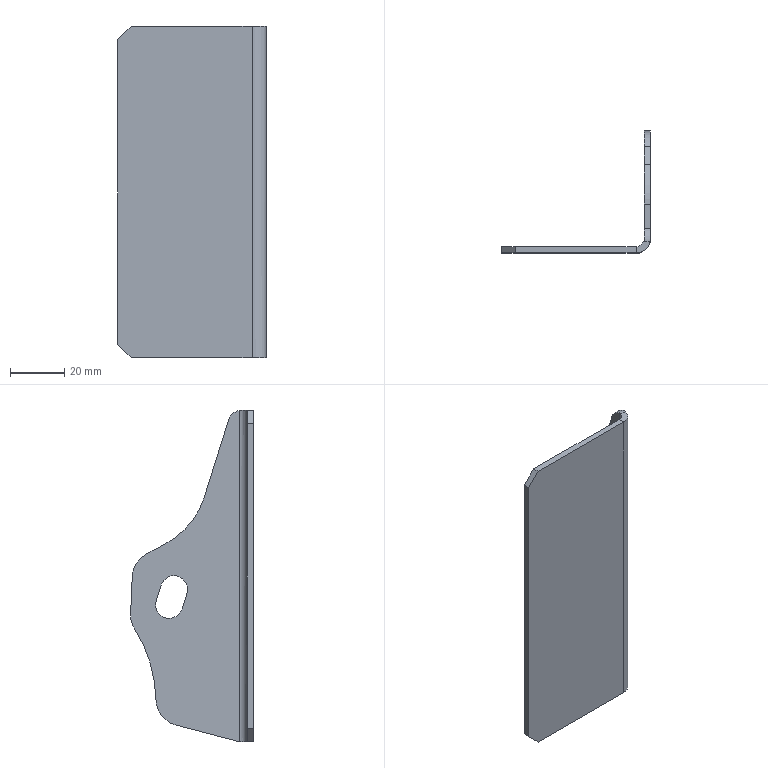Part | SolidWorks | features Chamfer 1, Fillet 1, FlatPattern 1, ICE 1, SMBaseFlange 1, SheetMetal 1 | 1 solid | 29 faces | box 55 x 45.365 x 122.5 mm | volume 22297 mm3 | plane 17 | cylinder 12 | commonest cylinder face diameters 10 x5 20 x3 6 x1 10.6 x1 60 x1 100 x1
STEP:
#1=CARTESIAN_POINT('',(0.,29.298,0.1113));
#2=VERTEX_POINT('',#1);
#3=CARTESIAN_POINT('',(0.,34.067,-3.386));
#4=VERTEX_POINT('',#3);
#5=CARTESIAN_POINT('',(0.,29.298,-4.889));
#6=DIRECTION('',(-1.,0.,0.));
#7=DIRECTION('',(0.,0.,1.));
#8=AXIS2_PLACEMENT_3D('',#5,#6,#7);
#9=CIRCLE('',#8,5.);
#10=EDGE_CURVE('',#2,#4,#9,.T.);
#11=ORIENTED_EDGE('',*,*,#10,.F.);
#12=CARTESIAN_POINT('',(-2.3,29.298,0.1113));
#13=VERTEX_POINT('',#12);
#14=CARTESIAN_POINT('',(-2.3,29.298,0.1113));
#15=DIRECTION('',(-1.,0.,0.));
#16=VECTOR('',#15,1000.);
#17=LINE('',#14,#16);
#18=EDGE_CURVE('',#2,#13,#17,.T.);
#19=ORIENTED_EDGE('',*,*,#18,.T.);
#20=CARTESIAN_POINT('',(-2.3,34.067,-3.386));
#21=VERTEX_POINT('',#20);
#22=CARTESIAN_POINT('',(-2.3,29.298,-4.889));
#23=DIRECTION('',(-1.,0.,0.));
#24=DIRECTION('',(0.,0.,1.));
#25=AXIS2_PLACEMENT_3D('',#22,#23,#24);
#26=CIRCLE('',#25,5.);
#27=EDGE_CURVE('',#13,#21,#26,.T.);
#28=ORIENTED_EDGE('',*,*,#27,.T.);
#29=CARTESIAN_POINT('',(-2.3,34.067,-3.386));
#30=DIRECTION('',(1.,0.,0.));
#31=VECTOR('',#30,1000.);
#32=LINE('',#29,#31);
#33=EDGE_CURVE('',#21,#4,#32,.T.);
#34=ORIENTED_EDGE('',*,*,#33,.T.);
#35=EDGE_LOOP('',(#11,#19,#28,#34));
#36=FACE_OUTER_BOUND('',#35,.T.);
#37=CARTESIAN_POINT('',(-2.3,29.298,-4.889));
#38=DIRECTION('',(-1.,0.,0.));
#39=DIRECTION('',(0.,0.,1.));
#40=AXIS2_PLACEMENT_3D('',#37,#38,#39);
#41=CYLINDRICAL_SURFACE('',#40,5.);
#42=ADVANCED_FACE('',(#36),#41,.F.);
#43=CARTESIAN_POINT('',(-5.3,0.,61.25));
#44=VERTEX_POINT('',#43);
#45=CARTESIAN_POINT('',(-0.08895,4.333,61.25));
#46=VERTEX_POINT('',#45);
#47=CARTESIAN_POINT('',(-5.3,5.3,61.25));
#48=DIRECTION('',(0.,0.,1.));
#49=DIRECTION('',(-1.,0.,0.));
#50=AXIS2_PLACEMENT_3D('',#47,#48,#49);
#51=CIRCLE('',#50,5.3);
#52=EDGE_CURVE('',#44,#46,#51,.T.);
#53=ORIENTED_EDGE('',*,*,#52,.T.);
#54=CARTESIAN_POINT('',(-2.46,4.333,61.25));
#55=VERTEX_POINT('',#54);
#56=CARTESIAN_POINT('',(-5.3,4.333,61.25));
#57=DIRECTION('',(-1.,0.,0.));
#58=VECTOR('',#57,1000.);
#59=LINE('',#56,#58);
#60=EDGE_CURVE('',#46,#55,#59,.T.);
#61=ORIENTED_EDGE('',*,*,#60,.T.);
#62=CARTESIAN_POINT('',(-5.3,2.3,61.25));
#63=VERTEX_POINT('',#62);
#64=CARTESIAN_POINT('',(-5.3,5.3,61.25));
#65=DIRECTION('',(0.,0.,1.));
#66=DIRECTION('',(1.,0.,0.));
#67=AXIS2_PLACEMENT_3D('',#64,#65,#66);
#68=CIRCLE('',#67,3.);
#69=EDGE_CURVE('',#63,#55,#68,.T.);
#70=ORIENTED_EDGE('',*,*,#69,.F.);
#71=CARTESIAN_POINT('',(-5.3,0.,61.25));
#72=DIRECTION('',(0.,1.,0.));
#73=VECTOR('',#72,1000.);
#74=LINE('',#71,#73);
#75=EDGE_CURVE('',#44,#63,#74,.T.);
#76=ORIENTED_EDGE('',*,*,#75,.F.);
#77=EDGE_LOOP('',(#53,#61,#70,#76));
#78=FACE_OUTER_BOUND('',#77,.T.);
#79=CARTESIAN_POINT('',(-5.3,0.,61.25));
#80=DIRECTION('',(0.,0.,1.));
#81=DIRECTION('',(1.,0.,0.));
#82=AXIS2_PLACEMENT_3D('',#79,#80,#81);
#83=PLANE('',#82);
#84=ADVANCED_FACE('',(#78),#83,.T.);
#85=CARTESIAN_POINT('',(-50.,2.3,61.25));
#86=VERTEX_POINT('',#85);
#87=CARTESIAN_POINT('',(0.,2.3,61.25));
#88=DIRECTION('',(1.,0.,0.));
#89=VECTOR('',#88,1000.);
#90=LINE('',#87,#89);
#91=EDGE_CURVE('',#86,#63,#90,.T.);
#92=ORIENTED_EDGE('',*,*,#91,.F.);
#93=CARTESIAN_POINT('',(-50.,0.,61.25));
#94=VERTEX_POINT('',#93);
#95=CARTESIAN_POINT('',(-50.,5.3,61.25));
#96=DIRECTION('',(0.,-1.,0.));
#97=VECTOR('',#96,1000.);
#98=LINE('',#95,#97);
#99=EDGE_CURVE('',#86,#94,#98,.T.);
#100=ORIENTED_EDGE('',*,*,#99,.T.);
#101=CARTESIAN_POINT('',(0.,0.,61.25));
#102=DIRECTION('',(1.,0.,0.));
#103=VECTOR('',#102,1000.);
#104=LINE('',#101,#103);
#105=EDGE_CURVE('',#94,#44,#104,.T.);
#106=ORIENTED_EDGE('',*,*,#105,.T.);
#107=ORIENTED_EDGE('',*,*,#75,.T.);
#108=EDGE_LOOP('',(#92,#100,#106,#107));
#109=FACE_OUTER_BOUND('',#108,.T.);
#110=CARTESIAN_POINT('',(-2.3,5.3,61.25));
#111=DIRECTION('',(0.,0.,1.));
#112=DIRECTION('',(1.,0.,0.));
#113=AXIS2_PLACEMENT_3D('',#110,#111,#112);
#114=PLANE('',#113);
#115=ADVANCED_FACE('',(#109),#114,.T.);
#116=CARTESIAN_POINT('',(-5.3,2.3,-61.25));
#117=VERTEX_POINT('',#116);
#118=CARTESIAN_POINT('',(-2.371,4.652,-61.25));
#119=VERTEX_POINT('',#118);
#120=CARTESIAN_POINT('',(-5.3,5.3,-61.25));
#121=DIRECTION('',(0.,0.,1.));
#122=DIRECTION('',(1.,0.,0.));
#123=AXIS2_PLACEMENT_3D('',#120,#121,#122);
#124=CIRCLE('',#123,3.);
#125=EDGE_CURVE('',#117,#119,#124,.T.);
#126=ORIENTED_EDGE('',*,*,#125,.T.);
#127=CARTESIAN_POINT('',(-0.03977,4.652,-61.25));
#128=VERTEX_POINT('',#127);
#129=CARTESIAN_POINT('',(0.,4.652,-61.25));
#130=DIRECTION('',(1.,0.,0.));
#131=VECTOR('',#130,1000.);
#132=LINE('',#129,#131);
#133=EDGE_CURVE('',#119,#128,#132,.T.);
#134=ORIENTED_EDGE('',*,*,#133,.T.);
#135=CARTESIAN_POINT('',(-5.3,0.,-61.25));
#136=VERTEX_POINT('',#135);
#137=CARTESIAN_POINT('',(-5.3,5.3,-61.25));
#138=DIRECTION('',(0.,0.,1.));
#139=DIRECTION('',(-1.,0.,0.));
#140=AXIS2_PLACEMENT_3D('',#137,#138,#139);
#141=CIRCLE('',#140,5.3);
#142=EDGE_CURVE('',#136,#128,#141,.T.);
#143=ORIENTED_EDGE('',*,*,#142,.F.);
#144=CARTESIAN_POINT('',(-5.3,2.3,-61.25));
#145=DIRECTION('',(0.,-1.,0.));
#146=VECTOR('',#145,1000.);
#147=LINE('',#144,#146);
#148=EDGE_CURVE('',#117,#136,#147,.T.);
#149=ORIENTED_EDGE('',*,*,#148,.F.);
#150=EDGE_LOOP('',(#126,#134,#143,#149));
#151=FACE_OUTER_BOUND('',#150,.T.);
#152=CARTESIAN_POINT('',(0.,5.3,-61.25));
#153=DIRECTION('',(0.,0.,-1.));
#154=DIRECTION('',(-1.,0.,0.));
#155=AXIS2_PLACEMENT_3D('',#152,#153,#154);
#156=PLANE('',#155);
#157=ADVANCED_FACE('',(#151),#156,.T.);
#158=CARTESIAN_POINT('',(0.,5.3,61.156));
#159=VERTEX_POINT('',#158);
#160=CARTESIAN_POINT('',(0.,5.3,-61.208));
#161=VERTEX_POINT('',#160);
#162=CARTESIAN_POINT('',(0.,5.3,61.25));
#163=DIRECTION('',(0.,0.,-1.));
#164=VECTOR('',#163,1000.);
#165=LINE('',#162,#164);
#166=EDGE_CURVE('',#159,#161,#165,.T.);
#167=ORIENTED_EDGE('',*,*,#166,.T.);
#168=CARTESIAN_POINT('',(0.,5.927,-61.085));
#169=VERTEX_POINT('',#168);
#170=CARTESIAN_POINT('',(0.,4.652,-56.25));
#171=DIRECTION('',(1.,0.,0.));
#172=DIRECTION('',(0.,0.,1.));
#173=AXIS2_PLACEMENT_3D('',#170,#171,#172);
#174=CIRCLE('',#173,5.);
#175=EDGE_CURVE('',#161,#169,#174,.T.);
#176=ORIENTED_EDGE('',*,*,#175,.T.);
#177=CARTESIAN_POINT('',(0.,28.542,-55.122));
#178=VERTEX_POINT('',#177);
#179=CARTESIAN_POINT('',(0.,5.3,-61.25));
#180=DIRECTION('',(0.,0.967,0.255));
#181=VECTOR('',#180,1000.);
#182=LINE('',#179,#181);
#183=EDGE_CURVE('',#169,#178,#182,.T.);
#184=ORIENTED_EDGE('',*,*,#183,.T.);
#185=CARTESIAN_POINT('',(0.,35.991,-45.643));
#186=VERTEX_POINT('',#185);
#187=CARTESIAN_POINT('',(0.,25.993,-45.452));
#188=DIRECTION('',(1.,0.,0.));
#189=DIRECTION('',(0.,0.,-1.));
#190=AXIS2_PLACEMENT_3D('',#187,#188,#189);
#191=CIRCLE('',#190,10.);
#192=EDGE_CURVE('',#178,#186,#191,.T.);
#193=ORIENTED_EDGE('',*,*,#192,.T.);
#194=CARTESIAN_POINT('',(0.,43.801,-19.75));
#195=VERTEX_POINT('',#194);
#196=CARTESIAN_POINT('',(0.,85.982,-46.597));
#197=DIRECTION('',(-1.,0.,0.));
#198=DIRECTION('',(0.,0.,1.));
#199=AXIS2_PLACEMENT_3D('',#196,#197,#198);
#200=CIRCLE('',#199,50.);
#201=EDGE_CURVE('',#186,#195,#200,.T.);
#202=ORIENTED_EDGE('',*,*,#201,.T.);
#203=CARTESIAN_POINT('',(0.,45.355,-13.942));
#204=VERTEX_POINT('',#203);
#205=CARTESIAN_POINT('',(0.,35.365,-14.38));
#206=DIRECTION('',(1.,0.,0.));
#207=DIRECTION('',(0.,0.,-1.));
#208=AXIS2_PLACEMENT_3D('',#205,#206,#207);
#209=CIRCLE('',#208,10.);
#210=EDGE_CURVE('',#195,#204,#209,.T.);
#211=ORIENTED_EDGE('',*,*,#210,.T.);
#212=CARTESIAN_POINT('',(0.,44.752,-0.1975));
#213=VERTEX_POINT('',#212);
#214=CARTESIAN_POINT('',(0.,44.752,-0.1975));
#215=DIRECTION('',(0.,-0.04382,0.999));
#216=VECTOR('',#215,1000.);
#217=LINE('',#214,#216);
#218=EDGE_CURVE('',#204,#213,#217,.T.);
#219=ORIENTED_EDGE('',*,*,#218,.T.);
#220=CARTESIAN_POINT('',(0.,39.405,8.221));
#221=VERTEX_POINT('',#220);
#222=CARTESIAN_POINT('',(0.,34.762,-0.6357));
#223=DIRECTION('',(1.,0.,0.));
#224=DIRECTION('',(0.,0.,-1.));
#225=AXIS2_PLACEMENT_3D('',#222,#223,#224);
#226=CIRCLE('',#225,10.);
#227=EDGE_CURVE('',#213,#221,#226,.T.);
#228=ORIENTED_EDGE('',*,*,#227,.T.);
#229=CARTESIAN_POINT('',(0.,32.764,11.702));
#230=VERTEX_POINT('',#229);
#231=CARTESIAN_POINT('',(0.,32.764,11.702));
#232=DIRECTION('',(0.,-0.8857,0.4643));
#233=VECTOR('',#232,1000.);
#234=LINE('',#231,#233);
#235=EDGE_CURVE('',#221,#230,#234,.T.);
#236=ORIENTED_EDGE('',*,*,#235,.T.);
#237=CARTESIAN_POINT('',(0.,18.08,29.257));
#238=VERTEX_POINT('',#237);
#239=CARTESIAN_POINT('',(0.,46.693,38.273));
#240=DIRECTION('',(-1.,0.,0.));
#241=DIRECTION('',(0.,0.,1.));
#242=AXIS2_PLACEMENT_3D('',#239,#240,#241);
#243=CIRCLE('',#242,30.);
#244=EDGE_CURVE('',#230,#238,#243,.T.);
#245=ORIENTED_EDGE('',*,*,#244,.T.);
#246=CARTESIAN_POINT('',(0.,9.102,57.753));
#247=VERTEX_POINT('',#246);
#248=CARTESIAN_POINT('',(0.,18.08,29.257));
#249=DIRECTION('',(0.,-0.3005,0.9538));
#250=VECTOR('',#249,1000.);
#251=LINE('',#248,#250);
#252=EDGE_CURVE('',#238,#247,#251,.T.);
#253=ORIENTED_EDGE('',*,*,#252,.T.);
#254=CARTESIAN_POINT('',(0.,4.333,56.25));
#255=DIRECTION('',(1.,0.,0.));
#256=DIRECTION('',(0.,0.,1.));
#257=AXIS2_PLACEMENT_3D('',#254,#255,#256);
#258=CIRCLE('',#257,5.);
#259=EDGE_CURVE('',#247,#159,#258,.T.);
#260=ORIENTED_EDGE('',*,*,#259,.T.);
#261=EDGE_LOOP('',(#167,#176,#184,#193,#202,#211,#219,#228,#236,#245,#253,#260));
#262=FACE_OUTER_BOUND('',#261,.T.);
#263=CARTESIAN_POINT('',(0.,26.333,-12.114));
#264=VERTEX_POINT('',#263);
#265=CARTESIAN_POINT('',(0.,24.53,-6.391));
#266=VERTEX_POINT('',#265);
#267=CARTESIAN_POINT('',(0.,26.333,-12.114));
#268=DIRECTION('',(0.,-0.3005,0.9538));
#269=VECTOR('',#268,1000.);
#270=LINE('',#267,#269);
#271=EDGE_CURVE('',#264,#266,#270,.T.);
#272=ORIENTED_EDGE('',*,*,#271,.T.);
#273=CARTESIAN_POINT('',(0.,29.298,-4.889));
#274=DIRECTION('',(-1.,0.,0.));
#275=DIRECTION('',(0.,0.,1.));
#276=AXIS2_PLACEMENT_3D('',#273,#274,#275);
#277=CIRCLE('',#276,5.);
#278=EDGE_CURVE('',#266,#2,#277,.T.);
#279=ORIENTED_EDGE('',*,*,#278,.T.);
#280=ORIENTED_EDGE('',*,*,#10,.T.);
#281=CARTESIAN_POINT('',(0.,35.87,-9.109));
#282=VERTEX_POINT('',#281);
#283=CARTESIAN_POINT('',(0.,35.87,-9.109));
#284=DIRECTION('',(0.,0.3005,-0.9538));
#285=VECTOR('',#284,1000.);
#286=LINE('',#283,#285);
#287=EDGE_CURVE('',#4,#282,#286,.T.);
#288=ORIENTED_EDGE('',*,*,#287,.T.);
#289=CARTESIAN_POINT('',(0.,31.102,-10.611));
#290=DIRECTION('',(-1.,0.,0.));
#291=DIRECTION('',(0.,0.,1.));
#292=AXIS2_PLACEMENT_3D('',#289,#290,#291);
#293=CIRCLE('',#292,5.);
#294=EDGE_CURVE('',#282,#264,#293,.T.);
#295=ORIENTED_EDGE('',*,*,#294,.T.);
#296=EDGE_LOOP('',(#272,#279,#280,#288,#295));
#297=FACE_BOUND('',#296,.T.);
#298=CARTESIAN_POINT('',(0.,0.,61.25));
#299=DIRECTION('',(-1.,0.,0.));
#300=DIRECTION('',(0.,0.,1.));
#301=AXIS2_PLACEMENT_3D('',#298,#299,#300);
#302=PLANE('',#301);
#303=ADVANCED_FACE('',(#262,#297),#302,.F.);
#304=CARTESIAN_POINT('',(-2.3,24.53,-6.391));
#305=VERTEX_POINT('',#304);
#306=CARTESIAN_POINT('',(-2.3,29.298,-4.889));
#307=DIRECTION('',(-1.,0.,0.));
#308=DIRECTION('',(0.,0.,1.));
#309=AXIS2_PLACEMENT_3D('',#306,#307,#308);
#310=CIRCLE('',#309,5.);
#311=EDGE_CURVE('',#305,#13,#310,.T.);
#312=ORIENTED_EDGE('',*,*,#311,.F.);
#313=CARTESIAN_POINT('',(-2.3,26.333,-12.114));
#314=VERTEX_POINT('',#313);
#315=CARTESIAN_POINT('',(-2.3,26.333,-12.114));
#316=DIRECTION('',(0.,-0.3005,0.9538));
#317=VECTOR('',#316,1000.);
#318=LINE('',#315,#317);
#319=EDGE_CURVE('',#314,#305,#318,.T.);
#320=ORIENTED_EDGE('',*,*,#319,.F.);
#321=CARTESIAN_POINT('',(-2.3,35.87,-9.109));
#322=VERTEX_POINT('',#321);
#323=CARTESIAN_POINT('',(-2.3,31.102,-10.611));
#324=DIRECTION('',(-1.,0.,0.));
#325=DIRECTION('',(0.,0.,1.));
#326=AXIS2_PLACEMENT_3D('',#323,#324,#325);
#327=CIRCLE('',#326,5.);
#328=EDGE_CURVE('',#322,#314,#327,.T.);
#329=ORIENTED_EDGE('',*,*,#328,.F.);
#330=CARTESIAN_POINT('',(-2.3,35.87,-9.109));
#331=DIRECTION('',(0.,0.3005,-0.9538));
#332=VECTOR('',#331,1000.);
#333=LINE('',#330,#332);
#334=EDGE_CURVE('',#21,#322,#333,.T.);
#335=ORIENTED_EDGE('',*,*,#334,.F.);
#336=ORIENTED_EDGE('',*,*,#27,.F.);
#337=EDGE_LOOP('',(#312,#320,#329,#335,#336));
#338=FACE_BOUND('',#337,.T.);
#339=CARTESIAN_POINT('',(-2.3,5.927,-61.085));
#340=VERTEX_POINT('',#339);
#341=CARTESIAN_POINT('',(-2.3,28.542,-55.122));
#342=VERTEX_POINT('',#341);
#343=CARTESIAN_POINT('',(-2.3,5.3,-61.25));
#344=DIRECTION('',(0.,0.967,0.255));
#345=VECTOR('',#344,1000.);
#346=LINE('',#343,#345);
#347=EDGE_CURVE('',#340,#342,#346,.T.);
#348=ORIENTED_EDGE('',*,*,#347,.F.);
#349=CARTESIAN_POINT('',(-2.3,5.3,-61.208));
#350=VERTEX_POINT('',#349);
#351=CARTESIAN_POINT('',(-2.3,4.652,-56.25));
#352=DIRECTION('',(-1.,0.,0.));
#353=DIRECTION('',(0.,0.,1.));
#354=AXIS2_PLACEMENT_3D('',#351,#352,#353);
#355=CIRCLE('',#354,5.);
#356=EDGE_CURVE('',#340,#350,#355,.T.);
#357=ORIENTED_EDGE('',*,*,#356,.T.);
#358=CARTESIAN_POINT('',(-2.3,5.3,61.156));
#359=VERTEX_POINT('',#358);
#360=CARTESIAN_POINT('',(-2.3,5.3,61.25));
#361=DIRECTION('',(0.,0.,-1.));
#362=VECTOR('',#361,1000.);
#363=LINE('',#360,#362);
#364=EDGE_CURVE('',#359,#350,#363,.T.);
#365=ORIENTED_EDGE('',*,*,#364,.F.);
#366=CARTESIAN_POINT('',(-2.3,9.102,57.753));
#367=VERTEX_POINT('',#366);
#368=CARTESIAN_POINT('',(-2.3,4.333,56.25));
#369=DIRECTION('',(-1.,0.,0.));
#370=DIRECTION('',(0.,0.,1.));
#371=AXIS2_PLACEMENT_3D('',#368,#369,#370);
#372=CIRCLE('',#371,5.);
#373=EDGE_CURVE('',#359,#367,#372,.T.);
#374=ORIENTED_EDGE('',*,*,#373,.T.);
#375=CARTESIAN_POINT('',(-2.3,18.08,29.257));
#376=VERTEX_POINT('',#375);
#377=CARTESIAN_POINT('',(-2.3,18.08,29.257));
#378=DIRECTION('',(0.,-0.3005,0.9538));
#379=VECTOR('',#378,1000.);
#380=LINE('',#377,#379);
#381=EDGE_CURVE('',#376,#367,#380,.T.);
#382=ORIENTED_EDGE('',*,*,#381,.F.);
#383=CARTESIAN_POINT('',(-2.3,32.764,11.702));
#384=VERTEX_POINT('',#383);
#385=CARTESIAN_POINT('',(-2.3,46.693,38.273));
#386=DIRECTION('',(-1.,0.,0.));
#387=DIRECTION('',(0.,0.,1.));
#388=AXIS2_PLACEMENT_3D('',#385,#386,#387);
#389=CIRCLE('',#388,30.);
#390=EDGE_CURVE('',#384,#376,#389,.T.);
#391=ORIENTED_EDGE('',*,*,#390,.F.);
#392=CARTESIAN_POINT('',(-2.3,39.405,8.221));
#393=VERTEX_POINT('',#392);
#394=CARTESIAN_POINT('',(-2.3,32.764,11.702));
#395=DIRECTION('',(0.,-0.8857,0.4643));
#396=VECTOR('',#395,1000.);
#397=LINE('',#394,#396);
#398=EDGE_CURVE('',#393,#384,#397,.T.);
#399=ORIENTED_EDGE('',*,*,#398,.F.);
#400=CARTESIAN_POINT('',(-2.3,44.752,-0.1975));
#401=VERTEX_POINT('',#400);
#402=CARTESIAN_POINT('',(-2.3,34.762,-0.6357));
#403=DIRECTION('',(1.,0.,0.));
#404=DIRECTION('',(0.,0.,-1.));
#405=AXIS2_PLACEMENT_3D('',#402,#403,#404);
#406=CIRCLE('',#405,10.);
#407=EDGE_CURVE('',#401,#393,#406,.T.);
#408=ORIENTED_EDGE('',*,*,#407,.F.);
#409=CARTESIAN_POINT('',(-2.3,45.355,-13.942));
#410=VERTEX_POINT('',#409);
#411=CARTESIAN_POINT('',(-2.3,44.752,-0.1975));
#412=DIRECTION('',(0.,-0.04382,0.999));
#413=VECTOR('',#412,1000.);
#414=LINE('',#411,#413);
#415=EDGE_CURVE('',#410,#401,#414,.T.);
#416=ORIENTED_EDGE('',*,*,#415,.F.);
#417=CARTESIAN_POINT('',(-2.3,43.801,-19.75));
#418=VERTEX_POINT('',#417);
#419=CARTESIAN_POINT('',(-2.3,35.365,-14.38));
#420=DIRECTION('',(1.,0.,0.));
#421=DIRECTION('',(0.,0.,1.));
#422=AXIS2_PLACEMENT_3D('',#419,#420,#421);
#423=CIRCLE('',#422,10.);
#424=EDGE_CURVE('',#418,#410,#423,.T.);
#425=ORIENTED_EDGE('',*,*,#424,.F.);
#426=CARTESIAN_POINT('',(-2.3,35.991,-45.643));
#427=VERTEX_POINT('',#426);
#428=CARTESIAN_POINT('',(-2.3,85.982,-46.597));
#429=DIRECTION('',(-1.,0.,0.));
#430=DIRECTION('',(0.,0.,1.));
#431=AXIS2_PLACEMENT_3D('',#428,#429,#430);
#432=CIRCLE('',#431,50.);
#433=EDGE_CURVE('',#427,#418,#432,.T.);
#434=ORIENTED_EDGE('',*,*,#433,.F.);
#435=CARTESIAN_POINT('',(-2.3,25.993,-45.452));
#436=DIRECTION('',(1.,0.,0.));
#437=DIRECTION('',(0.,0.,-1.));
#438=AXIS2_PLACEMENT_3D('',#435,#436,#437);
#439=CIRCLE('',#438,10.);
#440=EDGE_CURVE('',#342,#427,#439,.T.);
#441=ORIENTED_EDGE('',*,*,#440,.F.);
#442=EDGE_LOOP('',(#348,#357,#365,#374,#382,#391,#399,#408,#416,#425,#434,#441));
#443=FACE_OUTER_BOUND('',#442,.T.);
#444=CARTESIAN_POINT('',(-2.3,0.,61.25));
#445=DIRECTION('',(-1.,0.,0.));
#446=DIRECTION('',(0.,0.,1.));
#447=AXIS2_PLACEMENT_3D('',#444,#445,#446);
#448=PLANE('',#447);
#449=ADVANCED_FACE('',(#338,#443),#448,.T.);
#450=ORIENTED_EDGE('',*,*,#364,.T.);
#451=CARTESIAN_POINT('',(-2.3,5.3,-61.208));
#452=CARTESIAN_POINT('',(-2.3,5.082,-61.236));
#453=CARTESIAN_POINT('',(-2.323,4.866,-61.25));
#454=CARTESIAN_POINT('',(-2.371,4.652,-61.25));
#455=B_SPLINE_CURVE_WITH_KNOTS('',3,(#451,#452,#453,#454),.UNSPECIFIED.,.F.,.F.,(4,4),(0.,0.0006533),.UNSPECIFIED.);
#456=EDGE_CURVE('',#350,#119,#455,.T.);
#457=ORIENTED_EDGE('',*,*,#456,.T.);
#458=ORIENTED_EDGE('',*,*,#125,.F.);
#459=CARTESIAN_POINT('',(-5.3,2.3,61.25));
#460=DIRECTION('',(0.,0.,-1.));
#461=VECTOR('',#460,1000.);
#462=LINE('',#459,#461);
#463=EDGE_CURVE('',#63,#117,#462,.T.);
#464=ORIENTED_EDGE('',*,*,#463,.F.);
#465=ORIENTED_EDGE('',*,*,#69,.T.);
#466=CARTESIAN_POINT('',(-2.46,4.333,61.25));
#467=CARTESIAN_POINT('',(-2.352,4.649,61.25));
#468=CARTESIAN_POINT('',(-2.3,4.972,61.22));
#469=CARTESIAN_POINT('',(-2.3,5.3,61.156));
#470=B_SPLINE_CURVE_WITH_KNOTS('',3,(#466,#467,#468,#469),.UNSPECIFIED.,.F.,.F.,(4,4),(0.,0.0009847),.UNSPECIFIED.);
#471=EDGE_CURVE('',#55,#359,#470,.T.);
#472=ORIENTED_EDGE('',*,*,#471,.T.);
#473=EDGE_LOOP('',(#450,#457,#458,#464,#465,#472));
#474=FACE_OUTER_BOUND('',#473,.T.);
#475=CARTESIAN_POINT('',(-5.3,5.3,61.25));
#476=DIRECTION('',(0.,0.,-1.));
#477=DIRECTION('',(-1.,0.,0.));
#478=AXIS2_PLACEMENT_3D('',#475,#476,#477);
#479=CYLINDRICAL_SURFACE('',#478,3.);
#480=ADVANCED_FACE('',(#474),#479,.F.);
#481=CARTESIAN_POINT('',(-55.,2.3,56.25));
#482=VERTEX_POINT('',#481);
#483=CARTESIAN_POINT('',(-55.,2.3,-56.25));
#484=VERTEX_POINT('',#483);
#485=CARTESIAN_POINT('',(-55.,2.3,61.25));
#486=DIRECTION('',(0.,0.,-1.));
#487=VECTOR('',#486,1000.);
#488=LINE('',#485,#487);
#489=EDGE_CURVE('',#482,#484,#488,.T.);
#490=ORIENTED_EDGE('',*,*,#489,.F.);
#491=CARTESIAN_POINT('',(-25.,2.3,86.25));
#492=DIRECTION('',(0.7071,0.,0.7071));
#493=VECTOR('',#492,1000.);
#494=LINE('',#491,#493);
#495=EDGE_CURVE('',#482,#86,#494,.T.);
#496=ORIENTED_EDGE('',*,*,#495,.T.);
#497=ORIENTED_EDGE('',*,*,#91,.T.);
#498=ORIENTED_EDGE('',*,*,#463,.T.);
#499=CARTESIAN_POINT('',(-50.,2.3,-61.25));
#500=VERTEX_POINT('',#499);
#501=CARTESIAN_POINT('',(0.,2.3,-61.25));
#502=DIRECTION('',(1.,0.,0.));
#503=VECTOR('',#502,1000.);
#504=LINE('',#501,#503);
#505=EDGE_CURVE('',#500,#117,#504,.T.);
#506=ORIENTED_EDGE('',*,*,#505,.F.);
#507=CARTESIAN_POINT('',(-86.25,2.3,-25.));
#508=DIRECTION('',(-0.7071,0.,0.7071));
#509=VECTOR('',#508,1000.);
#510=LINE('',#507,#509);
#511=EDGE_CURVE('',#500,#484,#510,.T.);
#512=ORIENTED_EDGE('',*,*,#511,.T.);
#513=EDGE_LOOP('',(#490,#496,#497,#498,#506,#512));
#514=FACE_OUTER_BOUND('',#513,.T.);
#515=CARTESIAN_POINT('',(0.,2.3,61.25));
#516=DIRECTION('',(0.,1.,0.));
#517=DIRECTION('',(-1.,0.,0.));
#518=AXIS2_PLACEMENT_3D('',#515,#516,#517);
#519=PLANE('',#518);
#520=ADVANCED_FACE('',(#514),#519,.T.);
#521=CARTESIAN_POINT('',(-55.,0.,56.25));
#522=VERTEX_POINT('',#521);
#523=CARTESIAN_POINT('',(-55.,0.,-56.25));
#524=VERTEX_POINT('',#523);
#525=CARTESIAN_POINT('',(-55.,0.,61.25));
#526=DIRECTION('',(0.,0.,-1.));
#527=VECTOR('',#526,1000.);
#528=LINE('',#525,#527);
#529=EDGE_CURVE('',#522,#524,#528,.T.);
#530=ORIENTED_EDGE('',*,*,#529,.F.);
#531=CARTESIAN_POINT('',(-55.,0.,56.25));
#532=DIRECTION('',(0.,1.,0.));
#533=VECTOR('',#532,1000.);
#534=LINE('',#531,#533);
#535=EDGE_CURVE('',#522,#482,#534,.T.);
#536=ORIENTED_EDGE('',*,*,#535,.T.);
#537=ORIENTED_EDGE('',*,*,#489,.T.);
#538=CARTESIAN_POINT('',(-55.,0.,-56.25));
#539=DIRECTION('',(0.,-1.,0.));
#540=VECTOR('',#539,1000.);
#541=LINE('',#538,#540);
#542=EDGE_CURVE('',#484,#524,#541,.T.);
#543=ORIENTED_EDGE('',*,*,#542,.T.);
#544=EDGE_LOOP('',(#530,#536,#537,#543));
#545=FACE_OUTER_BOUND('',#544,.T.);
#546=CARTESIAN_POINT('',(-55.,0.,61.25));
#547=DIRECTION('',(-1.,0.,0.));
#548=DIRECTION('',(0.,0.,1.));
#549=AXIS2_PLACEMENT_3D('',#546,#547,#548);
#550=PLANE('',#549);
#551=ADVANCED_FACE('',(#545),#550,.T.);
#552=ORIENTED_EDGE('',*,*,#105,.F.);
#553=CARTESIAN_POINT('',(-55.,0.,56.25));
#554=DIRECTION('',(-0.7071,0.,-0.7071));
#555=VECTOR('',#554,1000.);
#556=LINE('',#553,#555);
#557=EDGE_CURVE('',#94,#522,#556,.T.);
#558=ORIENTED_EDGE('',*,*,#557,.T.);
#559=ORIENTED_EDGE('',*,*,#529,.T.);
#560=CARTESIAN_POINT('',(-50.,0.,-61.25));
#561=VERTEX_POINT('',#560);
#562=CARTESIAN_POINT('',(-50.,0.,-61.25));
#563=DIRECTION('',(0.7071,0.,-0.7071));
#564=VECTOR('',#563,1000.);
#565=LINE('',#562,#564);
#566=EDGE_CURVE('',#524,#561,#565,.T.);
#567=ORIENTED_EDGE('',*,*,#566,.T.);
#568=CARTESIAN_POINT('',(0.,0.,-61.25));
#569=DIRECTION('',(1.,0.,0.));
#570=VECTOR('',#569,1000.);
#571=LINE('',#568,#570);
#572=EDGE_CURVE('',#561,#136,#571,.T.);
#573=ORIENTED_EDGE('',*,*,#572,.T.);
#574=CARTESIAN_POINT('',(-5.3,0.,61.25));
#575=DIRECTION('',(0.,0.,-1.));
#576=VECTOR('',#575,1000.);
#577=LINE('',#574,#576);
#578=EDGE_CURVE('',#44,#136,#577,.T.);
#579=ORIENTED_EDGE('',*,*,#578,.F.);
#580=EDGE_LOOP('',(#552,#558,#559,#567,#573,#579));
#581=FACE_OUTER_BOUND('',#580,.T.);
#582=CARTESIAN_POINT('',(0.,0.,61.25));
#583=DIRECTION('',(0.,1.,0.));
#584=DIRECTION('',(-1.,0.,0.));
#585=AXIS2_PLACEMENT_3D('',#582,#583,#584);
#586=PLANE('',#585);
#587=ADVANCED_FACE('',(#581),#586,.F.);
#588=ORIENTED_EDGE('',*,*,#142,.T.);
#589=CARTESIAN_POINT('',(-0.03977,4.652,-61.25));
#590=CARTESIAN_POINT('',(-0.01315,4.868,-61.25));
#591=CARTESIAN_POINT('',(0.,5.084,-61.236));
#592=CARTESIAN_POINT('',(0.,5.3,-61.208));
#593=B_SPLINE_CURVE_WITH_KNOTS('',3,(#589,#590,#591,#592),.UNSPECIFIED.,.F.,.F.,(4,4),(0.,0.0006507),.UNSPECIFIED.);
#594=EDGE_CURVE('',#128,#161,#593,.T.);
#595=ORIENTED_EDGE('',*,*,#594,.T.);
#596=ORIENTED_EDGE('',*,*,#166,.F.);
#597=CARTESIAN_POINT('',(0.,5.3,61.156));
#598=CARTESIAN_POINT('',(0.,4.978,61.219));
#599=CARTESIAN_POINT('',(-0.02909,4.656,61.25));
#600=CARTESIAN_POINT('',(-0.08895,4.333,61.25));
#601=B_SPLINE_CURVE_WITH_KNOTS('',3,(#597,#598,#599,#600),.UNSPECIFIED.,.F.,.F.,(4,4),(0.,0.0009756),.UNSPECIFIED.);
#602=EDGE_CURVE('',#159,#46,#601,.T.);
#603=ORIENTED_EDGE('',*,*,#602,.T.);
#604=ORIENTED_EDGE('',*,*,#52,.F.);
#605=ORIENTED_EDGE('',*,*,#578,.T.);
#606=EDGE_LOOP('',(#588,#595,#596,#603,#604,#605));
#607=FACE_OUTER_BOUND('',#606,.T.);
#608=CARTESIAN_POINT('',(-5.3,5.3,61.25));
#609=DIRECTION('',(0.,0.,-1.));
#610=DIRECTION('',(-1.,0.,0.));
#611=AXIS2_PLACEMENT_3D('',#608,#609,#610);
#612=CYLINDRICAL_SURFACE('',#611,5.3);
#613=ADVANCED_FACE('',(#607),#612,.T.);
#614=ORIENTED_EDGE('',*,*,#572,.F.);
#615=CARTESIAN_POINT('',(-50.,2.3,-61.25));
#616=DIRECTION('',(0.,1.,0.));
#617=VECTOR('',#616,1000.);
#618=LINE('',#615,#617);
#619=EDGE_CURVE('',#561,#500,#618,.T.);
#620=ORIENTED_EDGE('',*,*,#619,.T.);
#621=ORIENTED_EDGE('',*,*,#505,.T.);
#622=ORIENTED_EDGE('',*,*,#148,.T.);
#623=EDGE_LOOP('',(#614,#620,#621,#622));
#624=FACE_OUTER_BOUND('',#623,.T.);
#625=CARTESIAN_POINT('',(-5.3,5.3,-61.25));
#626=DIRECTION('',(0.,0.,1.));
#627=DIRECTION('',(1.,0.,0.));
#628=AXIS2_PLACEMENT_3D('',#625,#626,#627);
#629=PLANE('',#628);
#630=ADVANCED_FACE('',(#624),#629,.F.);
#631=ORIENTED_EDGE('',*,*,#183,.F.);
#632=CARTESIAN_POINT('',(-2.3,5.927,-61.085));
#633=DIRECTION('',(-1.,0.,0.));
#634=VECTOR('',#633,1000.);
#635=LINE('',#632,#634);
#636=EDGE_CURVE('',#169,#340,#635,.T.);
#637=ORIENTED_EDGE('',*,*,#636,.T.);
#638=ORIENTED_EDGE('',*,*,#347,.T.);
#639=CARTESIAN_POINT('',(-2.3,28.542,-55.122));
#640=DIRECTION('',(1.,0.,0.));
#641=VECTOR('',#640,1000.);
#642=LINE('',#639,#641);
#643=EDGE_CURVE('',#342,#178,#642,.T.);
#644=ORIENTED_EDGE('',*,*,#643,.T.);
#645=EDGE_LOOP('',(#631,#637,#638,#644));
#646=FACE_OUTER_BOUND('',#645,.T.);
#647=CARTESIAN_POINT('',(-2.3,5.3,-61.25));
#648=DIRECTION('',(0.,-0.255,0.967));
#649=DIRECTION('',(0.,0.967,0.255));
#650=AXIS2_PLACEMENT_3D('',#647,#648,#649);
#651=PLANE('',#650);
#652=ADVANCED_FACE('',(#646),#651,.F.);
#653=ORIENTED_EDGE('',*,*,#643,.F.);
#654=ORIENTED_EDGE('',*,*,#440,.T.);
#655=CARTESIAN_POINT('',(-2.3,35.991,-45.643));
#656=DIRECTION('',(1.,0.,0.));
#657=VECTOR('',#656,1000.);
#658=LINE('',#655,#657);
#659=EDGE_CURVE('',#427,#186,#658,.T.);
#660=ORIENTED_EDGE('',*,*,#659,.T.);
#661=ORIENTED_EDGE('',*,*,#192,.F.);
#662=EDGE_LOOP('',(#653,#654,#660,#661));
#663=FACE_OUTER_BOUND('',#662,.T.);
#664=CARTESIAN_POINT('',(-2.3,25.993,-45.452));
#665=DIRECTION('',(-1.,0.,0.));
#666=DIRECTION('',(0.,0.,1.));
#667=AXIS2_PLACEMENT_3D('',#664,#665,#666);
#668=CYLINDRICAL_SURFACE('',#667,10.);
#669=ADVANCED_FACE('',(#663),#668,.T.);
#670=ORIENTED_EDGE('',*,*,#659,.F.);
#671=ORIENTED_EDGE('',*,*,#433,.T.);
#672=CARTESIAN_POINT('',(-2.3,43.801,-19.75));
#673=DIRECTION('',(1.,0.,0.));
#674=VECTOR('',#673,1000.);
#675=LINE('',#672,#674);
#676=EDGE_CURVE('',#418,#195,#675,.T.);
#677=ORIENTED_EDGE('',*,*,#676,.T.);
#678=ORIENTED_EDGE('',*,*,#201,.F.);
#679=EDGE_LOOP('',(#670,#671,#677,#678));
#680=FACE_OUTER_BOUND('',#679,.T.);
#681=CARTESIAN_POINT('',(-2.3,85.982,-46.597));
#682=DIRECTION('',(-1.,0.,0.));
#683=DIRECTION('',(0.,0.,1.));
#684=AXIS2_PLACEMENT_3D('',#681,#682,#683);
#685=CYLINDRICAL_SURFACE('',#684,50.);
#686=ADVANCED_FACE('',(#680),#685,.F.);
#687=ORIENTED_EDGE('',*,*,#676,.F.);
#688=ORIENTED_EDGE('',*,*,#424,.T.);
#689=CARTESIAN_POINT('',(-2.3,45.355,-13.942));
#690=DIRECTION('',(1.,0.,0.));
#691=VECTOR('',#690,1000.);
#692=LINE('',#689,#691);
#693=EDGE_CURVE('',#410,#204,#692,.T.);
#694=ORIENTED_EDGE('',*,*,#693,.T.);
#695=ORIENTED_EDGE('',*,*,#210,.F.);
#696=EDGE_LOOP('',(#687,#688,#694,#695));
#697=FACE_OUTER_BOUND('',#696,.T.);
#698=CARTESIAN_POINT('',(-2.3,35.365,-14.38));
#699=DIRECTION('',(-1.,0.,0.));
#700=DIRECTION('',(0.,0.,1.));
#701=AXIS2_PLACEMENT_3D('',#698,#699,#700);
#702=CYLINDRICAL_SURFACE('',#701,10.);
#703=ADVANCED_FACE('',(#697),#702,.T.);
#704=ORIENTED_EDGE('',*,*,#693,.F.);
#705=ORIENTED_EDGE('',*,*,#415,.T.);
#706=CARTESIAN_POINT('',(-2.3,44.752,-0.1975));
#707=DIRECTION('',(1.,0.,0.));
#708=VECTOR('',#707,1000.);
#709=LINE('',#706,#708);
#710=EDGE_CURVE('',#401,#213,#709,.T.);
#711=ORIENTED_EDGE('',*,*,#710,.T.);
#712=ORIENTED_EDGE('',*,*,#218,.F.);
#713=EDGE_LOOP('',(#704,#705,#711,#712));
#714=FACE_OUTER_BOUND('',#713,.T.);
#715=CARTESIAN_POINT('',(-2.3,44.752,-0.1975));
#716=DIRECTION('',(0.,-0.999,-0.04382));
#717=DIRECTION('',(0.,-0.04382,0.999));
#718=AXIS2_PLACEMENT_3D('',#715,#716,#717);
#719=PLANE('',#718);
#720=ADVANCED_FACE('',(#714),#719,.F.);
#721=ORIENTED_EDGE('',*,*,#710,.F.);
#722=ORIENTED_EDGE('',*,*,#407,.T.);
#723=CARTESIAN_POINT('',(-2.3,39.405,8.221));
#724=DIRECTION('',(1.,0.,0.));
#725=VECTOR('',#724,1000.);
#726=LINE('',#723,#725);
#727=EDGE_CURVE('',#393,#221,#726,.T.);
#728=ORIENTED_EDGE('',*,*,#727,.T.);
#729=ORIENTED_EDGE('',*,*,#227,.F.);
#730=EDGE_LOOP('',(#721,#722,#728,#729));
#731=FACE_OUTER_BOUND('',#730,.T.);
#732=CARTESIAN_POINT('',(-2.3,34.762,-0.6357));
#733=DIRECTION('',(-1.,0.,0.));
#734=DIRECTION('',(0.,0.,1.));
#735=AXIS2_PLACEMENT_3D('',#732,#733,#734);
#736=CYLINDRICAL_SURFACE('',#735,10.);
#737=ADVANCED_FACE('',(#731),#736,.T.);
#738=ORIENTED_EDGE('',*,*,#727,.F.);
#739=ORIENTED_EDGE('',*,*,#398,.T.);
#740=CARTESIAN_POINT('',(-2.3,32.764,11.702));
#741=DIRECTION('',(1.,0.,0.));
#742=VECTOR('',#741,1000.);
#743=LINE('',#740,#742);
#744=EDGE_CURVE('',#384,#230,#743,.T.);
#745=ORIENTED_EDGE('',*,*,#744,.T.);
#746=ORIENTED_EDGE('',*,*,#235,.F.);
#747=EDGE_LOOP('',(#738,#739,#745,#746));
#748=FACE_OUTER_BOUND('',#747,.T.);
#749=CARTESIAN_POINT('',(-2.3,32.764,11.702));
#750=DIRECTION('',(0.,-0.4643,-0.8857));
#751=DIRECTION('',(0.,-0.8857,0.4643));
#752=AXIS2_PLACEMENT_3D('',#749,#750,#751);
#753=PLANE('',#752);
#754=ADVANCED_FACE('',(#748),#753,.F.);
#755=ORIENTED_EDGE('',*,*,#744,.F.);
#756=ORIENTED_EDGE('',*,*,#390,.T.);
#757=CARTESIAN_POINT('',(-2.3,18.08,29.257));
#758=DIRECTION('',(1.,0.,0.));
#759=VECTOR('',#758,1000.);
#760=LINE('',#757,#759);
#761=EDGE_CURVE('',#376,#238,#760,.T.);
#762=ORIENTED_EDGE('',*,*,#761,.T.);
#763=ORIENTED_EDGE('',*,*,#244,.F.);
#764=EDGE_LOOP('',(#755,#756,#762,#763));
#765=FACE_OUTER_BOUND('',#764,.T.);
#766=CARTESIAN_POINT('',(-2.3,46.693,38.273));
#767=DIRECTION('',(-1.,0.,0.));
#768=DIRECTION('',(0.,0.,1.));
#769=AXIS2_PLACEMENT_3D('',#766,#767,#768);
#770=CYLINDRICAL_SURFACE('',#769,30.);
#771=ADVANCED_FACE('',(#765),#770,.F.);
#772=ORIENTED_EDGE('',*,*,#381,.T.);
#773=CARTESIAN_POINT('',(-2.3,9.102,57.753));
#774=DIRECTION('',(1.,0.,0.));
#775=VECTOR('',#774,1000.);
#776=LINE('',#773,#775);
#777=EDGE_CURVE('',#367,#247,#776,.T.);
#778=ORIENTED_EDGE('',*,*,#777,.T.);
#779=ORIENTED_EDGE('',*,*,#252,.F.);
#780=ORIENTED_EDGE('',*,*,#761,.F.);
#781=EDGE_LOOP('',(#772,#778,#779,#780));
#782=FACE_OUTER_BOUND('',#781,.T.);
#783=CARTESIAN_POINT('',(-2.3,18.08,29.257));
#784=DIRECTION('',(0.,-0.9538,-0.3005));
#785=DIRECTION('',(0.,-0.3005,0.9538));
#786=AXIS2_PLACEMENT_3D('',#783,#784,#785);
#787=PLANE('',#786);
#788=ADVANCED_FACE('',(#782),#787,.F.);
#789=CARTESIAN_POINT('',(-2.3,26.333,-12.114));
#790=DIRECTION('',(1.,0.,0.));
#791=VECTOR('',#790,1000.);
#792=LINE('',#789,#791);
#793=EDGE_CURVE('',#314,#264,#792,.T.);
#794=ORIENTED_EDGE('',*,*,#793,.F.);
#795=ORIENTED_EDGE('',*,*,#319,.T.);
#796=CARTESIAN_POINT('',(-2.3,24.53,-6.391));
#797=DIRECTION('',(1.,0.,0.));
#798=VECTOR('',#797,1000.);
#799=LINE('',#796,#798);
#800=EDGE_CURVE('',#305,#266,#799,.T.);
#801=ORIENTED_EDGE('',*,*,#800,.T.);
#802=ORIENTED_EDGE('',*,*,#271,.F.);
#803=EDGE_LOOP('',(#794,#795,#801,#802));
#804=FACE_OUTER_BOUND('',#803,.T.);
#805=CARTESIAN_POINT('',(-2.3,26.333,-12.114));
#806=DIRECTION('',(0.,-0.9538,-0.3005));
#807=DIRECTION('',(0.,-0.3005,0.9538));
#808=AXIS2_PLACEMENT_3D('',#805,#806,#807);
#809=PLANE('',#808);
#810=ADVANCED_FACE('',(#804),#809,.F.);
#811=ORIENTED_EDGE('',*,*,#18,.F.);
#812=ORIENTED_EDGE('',*,*,#278,.F.);
#813=ORIENTED_EDGE('',*,*,#800,.F.);
#814=ORIENTED_EDGE('',*,*,#311,.T.);
#815=EDGE_LOOP('',(#811,#812,#813,#814));
#816=FACE_OUTER_BOUND('',#815,.T.);
#817=CARTESIAN_POINT('',(-2.3,29.298,-4.889));
#818=DIRECTION('',(-1.,0.,0.));
#819=DIRECTION('',(0.,0.,1.));
#820=AXIS2_PLACEMENT_3D('',#817,#818,#819);
#821=CYLINDRICAL_SURFACE('',#820,5.);
#822=ADVANCED_FACE('',(#816),#821,.F.);
#823=ORIENTED_EDGE('',*,*,#33,.F.);
#824=ORIENTED_EDGE('',*,*,#334,.T.);
#825=CARTESIAN_POINT('',(-2.3,35.87,-9.109));
#826=DIRECTION('',(1.,0.,0.));
#827=VECTOR('',#826,1000.);
#828=LINE('',#825,#827);
#829=EDGE_CURVE('',#322,#282,#828,.T.);
#830=ORIENTED_EDGE('',*,*,#829,.T.);
#831=ORIENTED_EDGE('',*,*,#287,.F.);
#832=EDGE_LOOP('',(#823,#824,#830,#831));
#833=FACE_OUTER_BOUND('',#832,.T.);
#834=CARTESIAN_POINT('',(-2.3,35.87,-9.109));
#835=DIRECTION('',(0.,0.9538,0.3005));
#836=DIRECTION('',(0.,0.3005,-0.9538));
#837=AXIS2_PLACEMENT_3D('',#834,#835,#836);
#838=PLANE('',#837);
#839=ADVANCED_FACE('',(#833),#838,.F.);
#840=ORIENTED_EDGE('',*,*,#328,.T.);
#841=ORIENTED_EDGE('',*,*,#793,.T.);
#842=ORIENTED_EDGE('',*,*,#294,.F.);
#843=ORIENTED_EDGE('',*,*,#829,.F.);
#844=EDGE_LOOP('',(#840,#841,#842,#843));
#845=FACE_OUTER_BOUND('',#844,.T.);
#846=CARTESIAN_POINT('',(-2.3,31.102,-10.611));
#847=DIRECTION('',(-1.,0.,0.));
#848=DIRECTION('',(0.,0.,1.));
#849=AXIS2_PLACEMENT_3D('',#846,#847,#848);
#850=CYLINDRICAL_SURFACE('',#849,5.);
#851=ADVANCED_FACE('',(#845),#850,.F.);
#852=ORIENTED_EDGE('',*,*,#594,.F.);
#853=ORIENTED_EDGE('',*,*,#133,.F.);
#854=ORIENTED_EDGE('',*,*,#456,.F.);
#855=ORIENTED_EDGE('',*,*,#356,.F.);
#856=ORIENTED_EDGE('',*,*,#636,.F.);
#857=ORIENTED_EDGE('',*,*,#175,.F.);
#858=EDGE_LOOP('',(#852,#853,#854,#855,#856,#857));
#859=FACE_OUTER_BOUND('',#858,.T.);
#860=CARTESIAN_POINT('',(-2.3,4.652,-56.25));
#861=DIRECTION('',(1.,0.,0.));
#862=DIRECTION('',(0.,0.,-1.));
#863=AXIS2_PLACEMENT_3D('',#860,#861,#862);
#864=CYLINDRICAL_SURFACE('',#863,5.);
#865=ADVANCED_FACE('',(#859),#864,.T.);
#866=ORIENTED_EDGE('',*,*,#471,.F.);
#867=ORIENTED_EDGE('',*,*,#60,.F.);
#868=ORIENTED_EDGE('',*,*,#602,.F.);
#869=ORIENTED_EDGE('',*,*,#259,.F.);
#870=ORIENTED_EDGE('',*,*,#777,.F.);
#871=ORIENTED_EDGE('',*,*,#373,.F.);
#872=EDGE_LOOP('',(#866,#867,#868,#869,#870,#871));
#873=FACE_OUTER_BOUND('',#872,.T.);
#874=CARTESIAN_POINT('',(-2.3,4.333,56.25));
#875=DIRECTION('',(-1.,0.,0.));
#876=DIRECTION('',(0.,0.,1.));
#877=AXIS2_PLACEMENT_3D('',#874,#875,#876);
#878=CYLINDRICAL_SURFACE('',#877,5.);
#879=ADVANCED_FACE('',(#873),#878,.T.);
#880=ORIENTED_EDGE('',*,*,#557,.F.);
#881=ORIENTED_EDGE('',*,*,#99,.F.);
#882=ORIENTED_EDGE('',*,*,#495,.F.);
#883=ORIENTED_EDGE('',*,*,#535,.F.);
#884=EDGE_LOOP('',(#880,#881,#882,#883));
#885=FACE_OUTER_BOUND('',#884,.T.);
#886=CARTESIAN_POINT('',(-55.,0.,56.25));
#887=DIRECTION('',(0.7071,0.,-0.7071));
#888=DIRECTION('',(0.,1.,0.));
#889=AXIS2_PLACEMENT_3D('',#886,#887,#888);
#890=PLANE('',#889);
#891=ADVANCED_FACE('',(#885),#890,.F.);
#892=ORIENTED_EDGE('',*,*,#566,.F.);
#893=ORIENTED_EDGE('',*,*,#542,.F.);
#894=ORIENTED_EDGE('',*,*,#511,.F.);
#895=ORIENTED_EDGE('',*,*,#619,.F.);
#896=EDGE_LOOP('',(#892,#893,#894,#895));
#897=FACE_OUTER_BOUND('',#896,.T.);
#898=CARTESIAN_POINT('',(-50.,5.3,-61.25));
#899=DIRECTION('',(-0.7071,0.,-0.7071));
#900=DIRECTION('',(0.,-1.,0.));
#901=AXIS2_PLACEMENT_3D('',#898,#899,#900);
#902=PLANE('',#901);
#903=ADVANCED_FACE('',(#897),#902,.T.);
#904=CLOSED_SHELL('',(#42,#84,#115,#157,#303,#449,#480,#520,#551,#587,#613,#630,#652,#669,#686,#703,#720,#737,#754,#771,#788,#810,#822,#839,#851,#865,#879,#891,#903));
#905=MANIFOLD_SOLID_BREP('',#904);
#906=CARTESIAN_POINT('',(0.,0.,0.));
#907=DIRECTION('',(0.,0.,1.));
#908=DIRECTION('',(1.,0.,0.));
#909=AXIS2_PLACEMENT_3D('',#906,#907,#908);
#910=(LENGTH_UNIT()NAMED_UNIT(*)SI_UNIT(.MILLI.,.METRE.));
#911=UNCERTAINTY_MEASURE_WITH_UNIT(LENGTH_MEASURE(0.00001),#910,'','');
#912=(NAMED_UNIT(*)PLANE_ANGLE_UNIT()SI_UNIT($,.RADIAN.));
#913=(NAMED_UNIT(*)SI_UNIT($,.STERADIAN.)SOLID_ANGLE_UNIT());
#914=(GEOMETRIC_REPRESENTATION_CONTEXT(3)GLOBAL_UNCERTAINTY_ASSIGNED_CONTEXT((#911))GLOBAL_UNIT_ASSIGNED_CONTEXT((#910,#912,#913))REPRESENTATION_CONTEXT('',''));
#915=ADVANCED_BREP_SHAPE_REPRESENTATION('',(#905,#909),#914);